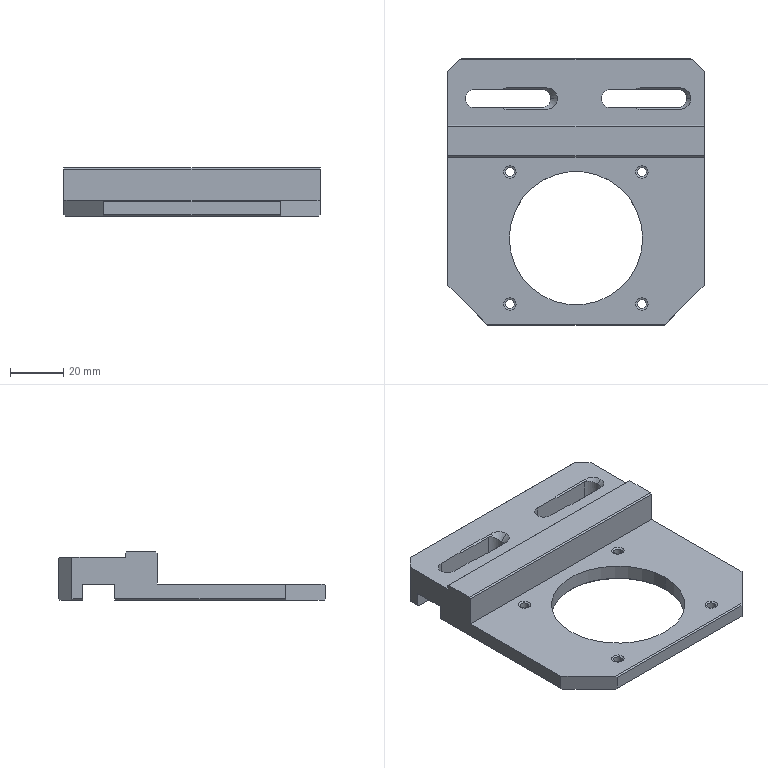Part | NX | 1 solid | 70 faces | box 96 x 100 x 18 mm | volume 70367 mm3 | plane 36 | cone 18 | cylinder 16 | commonest cylinder face diameters 3.3 x8 7 x6 50 x2